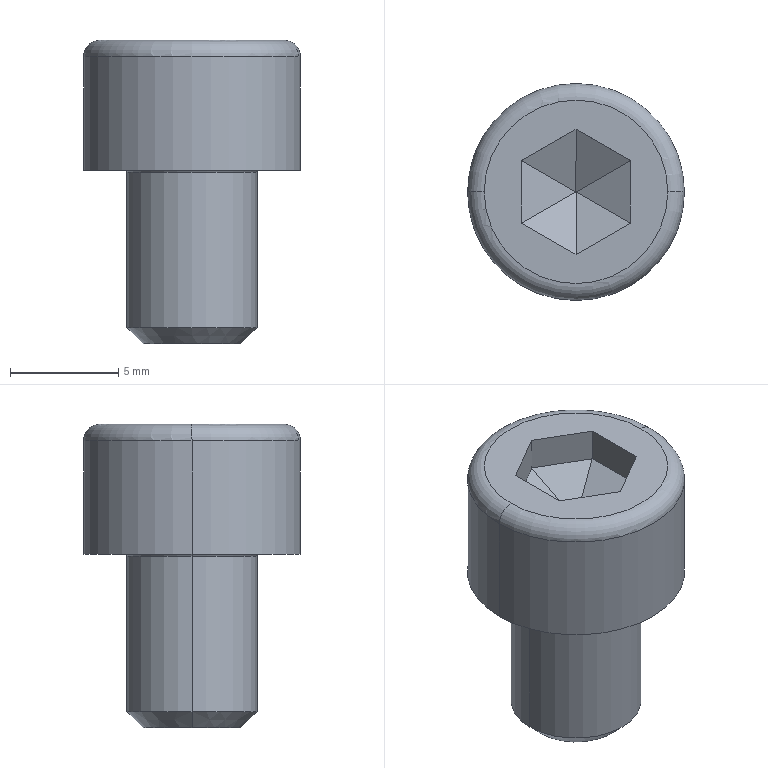Part | SolidWorks | features Chamfer 2, Fillet 2, ICE 2, Extrusion 1, RefAxis 1 | 1 solid | 26 faces | box 10 x 10 x 14 mm | volume 644.591 mm3 | plane 16 | torus 4 | cylinder 4 | cone 2 | commonest cylinder face diameters 6 x2 10 x2
STEP:
#1=CARTESIAN_POINT('',(-3.1,0.,0.));
#2=VERTEX_POINT('',#1);
#3=CARTESIAN_POINT('',(3.1,0.,0.));
#4=VERTEX_POINT('',#3);
#5=CARTESIAN_POINT('',(0.,0.,0.));
#6=DIRECTION('',(0.,0.,1.));
#7=DIRECTION('',(1.,0.,0.));
#8=AXIS2_PLACEMENT_3D('',#5,#6,#7);
#9=CIRCLE('',#8,3.1);
#10=EDGE_CURVE('',#2,#4,#9,.T.);
#11=ORIENTED_EDGE('',*,*,#10,.F.);
#12=CARTESIAN_POINT('',(-3.,0.,-0.1));
#13=VERTEX_POINT('',#12);
#14=CARTESIAN_POINT('',(-3.1,0.,-0.1));
#15=DIRECTION('',(0.,1.,0.));
#16=DIRECTION('',(-1.,0.,0.));
#17=AXIS2_PLACEMENT_3D('',#14,#15,#16);
#18=CIRCLE('',#17,0.1);
#19=EDGE_CURVE('',#2,#13,#18,.T.);
#20=ORIENTED_EDGE('',*,*,#19,.T.);
#21=CARTESIAN_POINT('',(3.,0.,-0.1));
#22=VERTEX_POINT('',#21);
#23=CARTESIAN_POINT('',(0.,0.,-0.1));
#24=DIRECTION('',(0.,0.,-1.));
#25=DIRECTION('',(1.,0.,0.));
#26=AXIS2_PLACEMENT_3D('',#23,#24,#25);
#27=CIRCLE('',#26,3.);
#28=EDGE_CURVE('',#22,#13,#27,.T.);
#29=ORIENTED_EDGE('',*,*,#28,.F.);
#30=CARTESIAN_POINT('',(3.1,0.,-0.1));
#31=DIRECTION('',(0.,-1.,0.));
#32=DIRECTION('',(0.,0.,-1.));
#33=AXIS2_PLACEMENT_3D('',#30,#31,#32);
#34=CIRCLE('',#33,0.1);
#35=EDGE_CURVE('',#4,#22,#34,.T.);
#36=ORIENTED_EDGE('',*,*,#35,.F.);
#37=EDGE_LOOP('',(#11,#20,#29,#36));
#38=FACE_OUTER_BOUND('',#37,.T.);
#39=CARTESIAN_POINT('',(0.,0.,-0.1));
#40=DIRECTION('',(0.,0.,1.));
#41=DIRECTION('',(1.,0.,0.));
#42=AXIS2_PLACEMENT_3D('',#39,#40,#41);
#43=TOROIDAL_SURFACE('',#42,3.1,0.1);
#44=ADVANCED_FACE('',(#38),#43,.F.);
#45=CARTESIAN_POINT('',(-5.,0.,5.231));
#46=VERTEX_POINT('',#45);
#47=CARTESIAN_POINT('',(5.,0.,5.231));
#48=VERTEX_POINT('',#47);
#49=CARTESIAN_POINT('',(0.,0.,5.231));
#50=DIRECTION('',(0.,0.,-1.));
#51=DIRECTION('',(1.,0.,0.));
#52=AXIS2_PLACEMENT_3D('',#49,#50,#51);
#53=CIRCLE('',#52,5.);
#54=EDGE_CURVE('',#46,#48,#53,.T.);
#55=ORIENTED_EDGE('',*,*,#54,.F.);
#56=CARTESIAN_POINT('',(-4.231,0.,6.));
#57=VERTEX_POINT('',#56);
#58=CARTESIAN_POINT('',(-4.231,0.,5.231));
#59=DIRECTION('',(0.,1.,0.));
#60=DIRECTION('',(-1.,0.,0.));
#61=AXIS2_PLACEMENT_3D('',#58,#59,#60);
#62=CIRCLE('',#61,0.7692);
#63=EDGE_CURVE('',#46,#57,#62,.T.);
#64=ORIENTED_EDGE('',*,*,#63,.T.);
#65=CARTESIAN_POINT('',(4.231,0.,6.));
#66=VERTEX_POINT('',#65);
#67=CARTESIAN_POINT('',(0.,0.,6.));
#68=DIRECTION('',(0.,0.,1.));
#69=DIRECTION('',(1.,0.,0.));
#70=AXIS2_PLACEMENT_3D('',#67,#68,#69);
#71=CIRCLE('',#70,4.231);
#72=EDGE_CURVE('',#66,#57,#71,.T.);
#73=ORIENTED_EDGE('',*,*,#72,.F.);
#74=CARTESIAN_POINT('',(4.231,0.,5.231));
#75=DIRECTION('',(0.,-1.,0.));
#76=DIRECTION('',(0.,0.,-1.));
#77=AXIS2_PLACEMENT_3D('',#74,#75,#76);
#78=CIRCLE('',#77,0.7692);
#79=EDGE_CURVE('',#48,#66,#78,.T.);
#80=ORIENTED_EDGE('',*,*,#79,.F.);
#81=EDGE_LOOP('',(#55,#64,#73,#80));
#82=FACE_OUTER_BOUND('',#81,.T.);
#83=CARTESIAN_POINT('',(0.,0.,5.231));
#84=DIRECTION('',(0.,0.,1.));
#85=DIRECTION('',(1.,0.,0.));
#86=AXIS2_PLACEMENT_3D('',#83,#84,#85);
#87=TOROIDAL_SURFACE('',#86,4.231,0.7692);
#88=ADVANCED_FACE('',(#82),#87,.T.);
#89=CARTESIAN_POINT('',(-2.25,0.,-8.));
#90=VERTEX_POINT('',#89);
#91=CARTESIAN_POINT('',(2.25,0.,-8.));
#92=VERTEX_POINT('',#91);
#93=CARTESIAN_POINT('',(0.,0.,-8.));
#94=DIRECTION('',(0.,0.,-1.));
#95=DIRECTION('',(-1.,0.,0.));
#96=AXIS2_PLACEMENT_3D('',#93,#94,#95);
#97=CIRCLE('',#96,2.25);
#98=EDGE_CURVE('',#90,#92,#97,.T.);
#99=ORIENTED_EDGE('',*,*,#98,.F.);
#100=CARTESIAN_POINT('',(-3.,0.,-7.25));
#101=VERTEX_POINT('',#100);
#102=CARTESIAN_POINT('',(-2.25,0.,-8.));
#103=DIRECTION('',(-0.7071,0.,0.7071));
#104=VECTOR('',#103,1000.);
#105=LINE('',#102,#104);
#106=EDGE_CURVE('',#90,#101,#105,.T.);
#107=ORIENTED_EDGE('',*,*,#106,.T.);
#108=CARTESIAN_POINT('',(3.,0.,-7.25));
#109=VERTEX_POINT('',#108);
#110=CARTESIAN_POINT('',(0.,0.,-7.25));
#111=DIRECTION('',(0.,0.,1.));
#112=DIRECTION('',(-1.,0.,0.));
#113=AXIS2_PLACEMENT_3D('',#110,#111,#112);
#114=CIRCLE('',#113,3.);
#115=EDGE_CURVE('',#109,#101,#114,.T.);
#116=ORIENTED_EDGE('',*,*,#115,.F.);
#117=CARTESIAN_POINT('',(2.25,0.,-8.));
#118=DIRECTION('',(0.7071,0.,0.7071));
#119=VECTOR('',#118,1000.);
#120=LINE('',#117,#119);
#121=EDGE_CURVE('',#92,#109,#120,.T.);
#122=ORIENTED_EDGE('',*,*,#121,.F.);
#123=EDGE_LOOP('',(#99,#107,#116,#122));
#124=FACE_OUTER_BOUND('',#123,.T.);
#125=CARTESIAN_POINT('',(0.,0.,-8.));
#126=DIRECTION('',(0.,0.,1.));
#127=DIRECTION('',(1.,0.,0.));
#128=AXIS2_PLACEMENT_3D('',#125,#126,#127);
#129=CONICAL_SURFACE('',#128,2.25,0.7854);
#130=ADVANCED_FACE('',(#124),#129,.T.);
#131=ORIENTED_EDGE('',*,*,#115,.T.);
#132=CARTESIAN_POINT('',(-3.,0.,-8.));
#133=DIRECTION('',(0.,0.,1.));
#134=VECTOR('',#133,1000.);
#135=LINE('',#132,#134);
#136=EDGE_CURVE('',#101,#13,#135,.T.);
#137=ORIENTED_EDGE('',*,*,#136,.T.);
#138=CARTESIAN_POINT('',(0.,0.,-0.1));
#139=DIRECTION('',(0.,0.,-1.));
#140=DIRECTION('',(1.,0.,0.));
#141=AXIS2_PLACEMENT_3D('',#138,#139,#140);
#142=CIRCLE('',#141,3.);
#143=EDGE_CURVE('',#13,#22,#142,.T.);
#144=ORIENTED_EDGE('',*,*,#143,.T.);
#145=CARTESIAN_POINT('',(3.,0.,-8.));
#146=DIRECTION('',(0.,0.,1.));
#147=VECTOR('',#146,1000.);
#148=LINE('',#145,#147);
#149=EDGE_CURVE('',#109,#22,#148,.T.);
#150=ORIENTED_EDGE('',*,*,#149,.F.);
#151=EDGE_LOOP('',(#131,#137,#144,#150));
#152=FACE_OUTER_BOUND('',#151,.T.);
#153=CARTESIAN_POINT('',(0.,0.,-8.));
#154=DIRECTION('',(0.,0.,1.));
#155=DIRECTION('',(1.,0.,0.));
#156=AXIS2_PLACEMENT_3D('',#153,#154,#155);
#157=CYLINDRICAL_SURFACE('',#156,3.);
#158=ADVANCED_FACE('',(#152),#157,.T.);
#159=ORIENTED_EDGE('',*,*,#54,.T.);
#160=CARTESIAN_POINT('',(5.,0.,0.));
#161=VERTEX_POINT('',#160);
#162=CARTESIAN_POINT('',(5.,0.,6.));
#163=DIRECTION('',(0.,0.,-1.));
#164=VECTOR('',#163,1000.);
#165=LINE('',#162,#164);
#166=EDGE_CURVE('',#48,#161,#165,.T.);
#167=ORIENTED_EDGE('',*,*,#166,.T.);
#168=CARTESIAN_POINT('',(-5.,0.,0.));
#169=VERTEX_POINT('',#168);
#170=CARTESIAN_POINT('',(0.,0.,0.));
#171=DIRECTION('',(0.,0.,1.));
#172=DIRECTION('',(1.,0.,0.));
#173=AXIS2_PLACEMENT_3D('',#170,#171,#172);
#174=CIRCLE('',#173,5.);
#175=EDGE_CURVE('',#161,#169,#174,.T.);
#176=ORIENTED_EDGE('',*,*,#175,.T.);
#177=CARTESIAN_POINT('',(-5.,0.,6.));
#178=DIRECTION('',(0.,0.,-1.));
#179=VECTOR('',#178,1000.);
#180=LINE('',#177,#179);
#181=EDGE_CURVE('',#46,#169,#180,.T.);
#182=ORIENTED_EDGE('',*,*,#181,.F.);
#183=EDGE_LOOP('',(#159,#167,#176,#182));
#184=FACE_OUTER_BOUND('',#183,.T.);
#185=CARTESIAN_POINT('',(0.,0.,6.));
#186=DIRECTION('',(0.,0.,-1.));
#187=DIRECTION('',(-1.,0.,0.));
#188=AXIS2_PLACEMENT_3D('',#185,#186,#187);
#189=CYLINDRICAL_SURFACE('',#188,5.);
#190=ADVANCED_FACE('',(#184),#189,.T.);
#191=CARTESIAN_POINT('',(0.,0.,0.));
#192=DIRECTION('',(0.,0.,1.));
#193=DIRECTION('',(1.,0.,0.));
#194=AXIS2_PLACEMENT_3D('',#191,#192,#193);
#195=CIRCLE('',#194,3.1);
#196=EDGE_CURVE('',#4,#2,#195,.T.);
#197=ORIENTED_EDGE('',*,*,#196,.T.);
#198=ORIENTED_EDGE('',*,*,#10,.T.);
#199=EDGE_LOOP('',(#197,#198));
#200=FACE_BOUND('',#199,.T.);
#201=CARTESIAN_POINT('',(0.,0.,0.));
#202=DIRECTION('',(0.,0.,1.));
#203=DIRECTION('',(1.,0.,0.));
#204=AXIS2_PLACEMENT_3D('',#201,#202,#203);
#205=CIRCLE('',#204,5.);
#206=EDGE_CURVE('',#169,#161,#205,.T.);
#207=ORIENTED_EDGE('',*,*,#206,.F.);
#208=ORIENTED_EDGE('',*,*,#175,.F.);
#209=EDGE_LOOP('',(#207,#208));
#210=FACE_OUTER_BOUND('',#209,.T.);
#211=CARTESIAN_POINT('',(0.,0.,0.));
#212=DIRECTION('',(0.,0.,1.));
#213=DIRECTION('',(1.,0.,0.));
#214=AXIS2_PLACEMENT_3D('',#211,#212,#213);
#215=PLANE('',#214);
#216=ADVANCED_FACE('',(#200,#210),#215,.F.);
#217=ORIENTED_EDGE('',*,*,#166,.F.);
#218=CARTESIAN_POINT('',(0.,0.,5.231));
#219=DIRECTION('',(0.,0.,-1.));
#220=DIRECTION('',(1.,0.,0.));
#221=AXIS2_PLACEMENT_3D('',#218,#219,#220);
#222=CIRCLE('',#221,5.);
#223=EDGE_CURVE('',#48,#46,#222,.T.);
#224=ORIENTED_EDGE('',*,*,#223,.T.);
#225=ORIENTED_EDGE('',*,*,#181,.T.);
#226=ORIENTED_EDGE('',*,*,#206,.T.);
#227=EDGE_LOOP('',(#217,#224,#225,#226));
#228=FACE_OUTER_BOUND('',#227,.T.);
#229=CARTESIAN_POINT('',(0.,0.,6.));
#230=DIRECTION('',(0.,0.,-1.));
#231=DIRECTION('',(-1.,0.,0.));
#232=AXIS2_PLACEMENT_3D('',#229,#230,#231);
#233=CYLINDRICAL_SURFACE('',#232,5.);
#234=ADVANCED_FACE('',(#228),#233,.T.);
#235=ORIENTED_EDGE('',*,*,#72,.T.);
#236=CARTESIAN_POINT('',(0.,0.,6.));
#237=DIRECTION('',(0.,0.,1.));
#238=DIRECTION('',(1.,0.,0.));
#239=AXIS2_PLACEMENT_3D('',#236,#237,#238);
#240=CIRCLE('',#239,4.231);
#241=EDGE_CURVE('',#57,#66,#240,.T.);
#242=ORIENTED_EDGE('',*,*,#241,.T.);
#243=EDGE_LOOP('',(#235,#242));
#244=FACE_OUTER_BOUND('',#243,.T.);
#245=CARTESIAN_POINT('',(2.5,-1.443,6.));
#246=VERTEX_POINT('',#245);
#247=CARTESIAN_POINT('',(2.5,1.443,6.));
#248=VERTEX_POINT('',#247);
#249=CARTESIAN_POINT('',(2.5,-1.443,6.));
#250=DIRECTION('',(0.,1.,0.));
#251=VECTOR('',#250,1000.);
#252=LINE('',#249,#251);
#253=EDGE_CURVE('',#246,#248,#252,.T.);
#254=ORIENTED_EDGE('',*,*,#253,.F.);
#255=CARTESIAN_POINT('',(0.,-2.887,6.));
#256=VERTEX_POINT('',#255);
#257=CARTESIAN_POINT('',(0.,-2.887,6.));
#258=DIRECTION('',(0.866,0.5,0.));
#259=VECTOR('',#258,1000.);
#260=LINE('',#257,#259);
#261=EDGE_CURVE('',#256,#246,#260,.T.);
#262=ORIENTED_EDGE('',*,*,#261,.F.);
#263=CARTESIAN_POINT('',(-2.5,-1.443,6.));
#264=VERTEX_POINT('',#263);
#265=CARTESIAN_POINT('',(-2.5,-1.443,6.));
#266=DIRECTION('',(0.866,-0.5,0.));
#267=VECTOR('',#266,1000.);
#268=LINE('',#265,#267);
#269=EDGE_CURVE('',#264,#256,#268,.T.);
#270=ORIENTED_EDGE('',*,*,#269,.F.);
#271=CARTESIAN_POINT('',(-2.5,1.443,6.));
#272=VERTEX_POINT('',#271);
#273=CARTESIAN_POINT('',(-2.5,1.443,6.));
#274=DIRECTION('',(0.,-1.,0.));
#275=VECTOR('',#274,1000.);
#276=LINE('',#273,#275);
#277=EDGE_CURVE('',#272,#264,#276,.T.);
#278=ORIENTED_EDGE('',*,*,#277,.F.);
#279=CARTESIAN_POINT('',(0.,2.887,6.));
#280=VERTEX_POINT('',#279);
#281=CARTESIAN_POINT('',(0.,2.887,6.));
#282=DIRECTION('',(-0.866,-0.5,0.));
#283=VECTOR('',#282,1000.);
#284=LINE('',#281,#283);
#285=EDGE_CURVE('',#280,#272,#284,.T.);
#286=ORIENTED_EDGE('',*,*,#285,.F.);
#287=CARTESIAN_POINT('',(2.5,1.443,6.));
#288=DIRECTION('',(-0.866,0.5,0.));
#289=VECTOR('',#288,1000.);
#290=LINE('',#287,#289);
#291=EDGE_CURVE('',#248,#280,#290,.T.);
#292=ORIENTED_EDGE('',*,*,#291,.F.);
#293=EDGE_LOOP('',(#254,#262,#270,#278,#286,#292));
#294=FACE_BOUND('',#293,.T.);
#295=CARTESIAN_POINT('',(0.,0.,6.));
#296=DIRECTION('',(0.,0.,1.));
#297=DIRECTION('',(1.,0.,0.));
#298=AXIS2_PLACEMENT_3D('',#295,#296,#297);
#299=PLANE('',#298);
#300=ADVANCED_FACE('',(#244,#294),#299,.T.);
#301=CARTESIAN_POINT('',(2.5,1.443,4.441));
#302=VERTEX_POINT('',#301);
#303=CARTESIAN_POINT('',(2.5,1.443,3.));
#304=DIRECTION('',(0.,0.,1.));
#305=VECTOR('',#304,1000.);
#306=LINE('',#303,#305);
#307=EDGE_CURVE('',#302,#248,#306,.T.);
#308=ORIENTED_EDGE('',*,*,#307,.F.);
#309=CARTESIAN_POINT('',(2.5,-1.443,4.441));
#310=VERTEX_POINT('',#309);
#311=CARTESIAN_POINT('',(2.5,-1.443,4.441));
#312=DIRECTION('',(0.,-1.,0.));
#313=VECTOR('',#312,1000.);
#314=LINE('',#311,#313);
#315=EDGE_CURVE('',#302,#310,#314,.T.);
#316=ORIENTED_EDGE('',*,*,#315,.T.);
#317=CARTESIAN_POINT('',(2.5,-1.443,3.));
#318=DIRECTION('',(0.,0.,1.));
#319=VECTOR('',#318,1000.);
#320=LINE('',#317,#319);
#321=EDGE_CURVE('',#310,#246,#320,.T.);
#322=ORIENTED_EDGE('',*,*,#321,.T.);
#323=ORIENTED_EDGE('',*,*,#253,.T.);
#324=EDGE_LOOP('',(#308,#316,#322,#323));
#325=FACE_OUTER_BOUND('',#324,.T.);
#326=CARTESIAN_POINT('',(2.5,-1.443,3.));
#327=DIRECTION('',(1.,0.,0.));
#328=DIRECTION('',(0.,0.,-1.));
#329=AXIS2_PLACEMENT_3D('',#326,#327,#328);
#330=PLANE('',#329);
#331=ADVANCED_FACE('',(#325),#330,.F.);
#332=ORIENTED_EDGE('',*,*,#321,.F.);
#333=CARTESIAN_POINT('',(0.,-2.887,4.441));
#334=VERTEX_POINT('',#333);
#335=CARTESIAN_POINT('',(0.,-2.887,4.441));
#336=DIRECTION('',(-0.866,-0.5,0.));
#337=VECTOR('',#336,1000.);
#338=LINE('',#335,#337);
#339=EDGE_CURVE('',#310,#334,#338,.T.);
#340=ORIENTED_EDGE('',*,*,#339,.T.);
#341=CARTESIAN_POINT('',(0.,-2.887,3.));
#342=DIRECTION('',(0.,0.,1.));
#343=VECTOR('',#342,1000.);
#344=LINE('',#341,#343);
#345=EDGE_CURVE('',#334,#256,#344,.T.);
#346=ORIENTED_EDGE('',*,*,#345,.T.);
#347=ORIENTED_EDGE('',*,*,#261,.T.);
#348=EDGE_LOOP('',(#332,#340,#346,#347));
#349=FACE_OUTER_BOUND('',#348,.T.);
#350=CARTESIAN_POINT('',(0.,-2.887,3.));
#351=DIRECTION('',(0.5,-0.866,0.));
#352=DIRECTION('',(0.866,0.5,0.));
#353=AXIS2_PLACEMENT_3D('',#350,#351,#352);
#354=PLANE('',#353);
#355=ADVANCED_FACE('',(#349),#354,.F.);
#356=ORIENTED_EDGE('',*,*,#345,.F.);
#357=CARTESIAN_POINT('',(-2.5,-1.443,4.441));
#358=VERTEX_POINT('',#357);
#359=CARTESIAN_POINT('',(-2.5,-1.443,4.441));
#360=DIRECTION('',(-0.866,0.5,0.));
#361=VECTOR('',#360,1000.);
#362=LINE('',#359,#361);
#363=EDGE_CURVE('',#334,#358,#362,.T.);
#364=ORIENTED_EDGE('',*,*,#363,.T.);
#365=CARTESIAN_POINT('',(-2.5,-1.443,3.));
#366=DIRECTION('',(0.,0.,1.));
#367=VECTOR('',#366,1000.);
#368=LINE('',#365,#367);
#369=EDGE_CURVE('',#358,#264,#368,.T.);
#370=ORIENTED_EDGE('',*,*,#369,.T.);
#371=ORIENTED_EDGE('',*,*,#269,.T.);
#372=EDGE_LOOP('',(#356,#364,#370,#371));
#373=FACE_OUTER_BOUND('',#372,.T.);
#374=CARTESIAN_POINT('',(-2.5,-1.443,3.));
#375=DIRECTION('',(-0.5,-0.866,0.));
#376=DIRECTION('',(0.866,-0.5,0.));
#377=AXIS2_PLACEMENT_3D('',#374,#375,#376);
#378=PLANE('',#377);
#379=ADVANCED_FACE('',(#373),#378,.F.);
#380=ORIENTED_EDGE('',*,*,#369,.F.);
#381=CARTESIAN_POINT('',(-2.5,1.443,4.441));
#382=VERTEX_POINT('',#381);
#383=CARTESIAN_POINT('',(-2.5,1.443,4.441));
#384=DIRECTION('',(0.,1.,0.));
#385=VECTOR('',#384,1000.);
#386=LINE('',#383,#385);
#387=EDGE_CURVE('',#358,#382,#386,.T.);
#388=ORIENTED_EDGE('',*,*,#387,.T.);
#389=CARTESIAN_POINT('',(-2.5,1.443,3.));
#390=DIRECTION('',(0.,0.,1.));
#391=VECTOR('',#390,1000.);
#392=LINE('',#389,#391);
#393=EDGE_CURVE('',#382,#272,#392,.T.);
#394=ORIENTED_EDGE('',*,*,#393,.T.);
#395=ORIENTED_EDGE('',*,*,#277,.T.);
#396=EDGE_LOOP('',(#380,#388,#394,#395));
#397=FACE_OUTER_BOUND('',#396,.T.);
#398=CARTESIAN_POINT('',(-2.5,1.443,3.));
#399=DIRECTION('',(-1.,0.,0.));
#400=DIRECTION('',(0.,0.,1.));
#401=AXIS2_PLACEMENT_3D('',#398,#399,#400);
#402=PLANE('',#401);
#403=ADVANCED_FACE('',(#397),#402,.F.);
#404=ORIENTED_EDGE('',*,*,#393,.F.);
#405=CARTESIAN_POINT('',(0.,2.887,4.441));
#406=VERTEX_POINT('',#405);
#407=CARTESIAN_POINT('',(0.,2.887,4.441));
#408=DIRECTION('',(0.866,0.5,0.));
#409=VECTOR('',#408,1000.);
#410=LINE('',#407,#409);
#411=EDGE_CURVE('',#382,#406,#410,.T.);
#412=ORIENTED_EDGE('',*,*,#411,.T.);
#413=CARTESIAN_POINT('',(0.,2.887,3.));
#414=DIRECTION('',(0.,0.,1.));
#415=VECTOR('',#414,1000.);
#416=LINE('',#413,#415);
#417=EDGE_CURVE('',#406,#280,#416,.T.);
#418=ORIENTED_EDGE('',*,*,#417,.T.);
#419=ORIENTED_EDGE('',*,*,#285,.T.);
#420=EDGE_LOOP('',(#404,#412,#418,#419));
#421=FACE_OUTER_BOUND('',#420,.T.);
#422=CARTESIAN_POINT('',(0.,2.887,3.));
#423=DIRECTION('',(-0.5,0.866,0.));
#424=DIRECTION('',(-0.866,-0.5,0.));
#425=AXIS2_PLACEMENT_3D('',#422,#423,#424);
#426=PLANE('',#425);
#427=ADVANCED_FACE('',(#421),#426,.F.);
#428=ORIENTED_EDGE('',*,*,#417,.F.);
#429=CARTESIAN_POINT('',(2.5,1.443,4.441));
#430=DIRECTION('',(0.866,-0.5,0.));
#431=VECTOR('',#430,1000.);
#432=LINE('',#429,#431);
#433=EDGE_CURVE('',#406,#302,#432,.T.);
#434=ORIENTED_EDGE('',*,*,#433,.T.);
#435=ORIENTED_EDGE('',*,*,#307,.T.);
#436=ORIENTED_EDGE('',*,*,#291,.T.);
#437=EDGE_LOOP('',(#428,#434,#435,#436));
#438=FACE_OUTER_BOUND('',#437,.T.);
#439=CARTESIAN_POINT('',(2.5,1.443,3.));
#440=DIRECTION('',(0.5,0.866,0.));
#441=DIRECTION('',(-0.866,0.5,0.));
#442=AXIS2_PLACEMENT_3D('',#439,#440,#441);
#443=PLANE('',#442);
#444=ADVANCED_FACE('',(#438),#443,.F.);
#445=CARTESIAN_POINT('',(0.,0.004907,3.));
#446=VERTEX_POINT('',#445);
#447=CARTESIAN_POINT('',(-0.00425,0.002453,3.));
#448=VERTEX_POINT('',#447);
#449=CARTESIAN_POINT('',(-0.002125,0.00368,3.));
#450=DIRECTION('',(-0.866,-0.5,0.));
#451=VECTOR('',#450,1000.);
#452=LINE('',#449,#451);
#453=EDGE_CURVE('',#446,#448,#452,.T.);
#454=ORIENTED_EDGE('',*,*,#453,.T.);
#455=CARTESIAN_POINT('',(-0.00425,-0.002453,3.));
#456=VERTEX_POINT('',#455);
#457=CARTESIAN_POINT('',(-0.00425,0.,3.));
#458=DIRECTION('',(0.,-1.,0.));
#459=VECTOR('',#458,1000.);
#460=LINE('',#457,#459);
#461=EDGE_CURVE('',#448,#456,#460,.T.);
#462=ORIENTED_EDGE('',*,*,#461,.T.);
#463=CARTESIAN_POINT('',(0.,-0.004907,3.));
#464=VERTEX_POINT('',#463);
#465=CARTESIAN_POINT('',(-0.002125,-0.00368,3.));
#466=DIRECTION('',(0.866,-0.5,0.));
#467=VECTOR('',#466,1000.);
#468=LINE('',#465,#467);
#469=EDGE_CURVE('',#456,#464,#468,.T.);
#470=ORIENTED_EDGE('',*,*,#469,.T.);
#471=CARTESIAN_POINT('',(0.00425,-0.002453,3.));
#472=VERTEX_POINT('',#471);
#473=CARTESIAN_POINT('',(0.002125,-0.00368,3.));
#474=DIRECTION('',(0.866,0.5,0.));
#475=VECTOR('',#474,1000.);
#476=LINE('',#473,#475);
#477=EDGE_CURVE('',#464,#472,#476,.T.);
#478=ORIENTED_EDGE('',*,*,#477,.T.);
#479=CARTESIAN_POINT('',(0.00425,0.002453,3.));
#480=VERTEX_POINT('',#479);
#481=CARTESIAN_POINT('',(0.00425,0.,3.));
#482=DIRECTION('',(0.,1.,0.));
#483=VECTOR('',#482,1000.);
#484=LINE('',#481,#483);
#485=EDGE_CURVE('',#472,#480,#484,.T.);
#486=ORIENTED_EDGE('',*,*,#485,.T.);
#487=CARTESIAN_POINT('',(0.002125,0.00368,3.));
#488=DIRECTION('',(-0.866,0.5,0.));
#489=VECTOR('',#488,1000.);
#490=LINE('',#487,#489);
#491=EDGE_CURVE('',#480,#446,#490,.T.);
#492=ORIENTED_EDGE('',*,*,#491,.T.);
#493=EDGE_LOOP('',(#454,#462,#470,#478,#486,#492));
#494=FACE_OUTER_BOUND('',#493,.T.);
#495=CARTESIAN_POINT('',(0.,0.,3.));
#496=DIRECTION('',(0.,0.,1.));
#497=DIRECTION('',(1.,0.,0.));
#498=AXIS2_PLACEMENT_3D('',#495,#496,#497);
#499=PLANE('',#498);
#500=ADVANCED_FACE('',(#494),#499,.T.);
#501=ORIENTED_EDGE('',*,*,#136,.F.);
#502=CARTESIAN_POINT('',(0.,0.,-7.25));
#503=DIRECTION('',(0.,0.,1.));
#504=DIRECTION('',(-1.,0.,0.));
#505=AXIS2_PLACEMENT_3D('',#502,#503,#504);
#506=CIRCLE('',#505,3.);
#507=EDGE_CURVE('',#101,#109,#506,.T.);
#508=ORIENTED_EDGE('',*,*,#507,.T.);
#509=ORIENTED_EDGE('',*,*,#149,.T.);
#510=ORIENTED_EDGE('',*,*,#28,.T.);
#511=EDGE_LOOP('',(#501,#508,#509,#510));
#512=FACE_OUTER_BOUND('',#511,.T.);
#513=CARTESIAN_POINT('',(0.,0.,-8.));
#514=DIRECTION('',(0.,0.,1.));
#515=DIRECTION('',(1.,0.,0.));
#516=AXIS2_PLACEMENT_3D('',#513,#514,#515);
#517=CYLINDRICAL_SURFACE('',#516,3.);
#518=ADVANCED_FACE('',(#512),#517,.T.);
#519=CARTESIAN_POINT('',(0.,0.,-8.));
#520=DIRECTION('',(0.,0.,-1.));
#521=DIRECTION('',(-1.,0.,0.));
#522=AXIS2_PLACEMENT_3D('',#519,#520,#521);
#523=CIRCLE('',#522,2.25);
#524=EDGE_CURVE('',#92,#90,#523,.T.);
#525=ORIENTED_EDGE('',*,*,#524,.T.);
#526=ORIENTED_EDGE('',*,*,#98,.T.);
#527=EDGE_LOOP('',(#525,#526));
#528=FACE_OUTER_BOUND('',#527,.T.);
#529=CARTESIAN_POINT('',(0.,0.,-8.));
#530=DIRECTION('',(0.,0.,-1.));
#531=DIRECTION('',(-1.,0.,0.));
#532=AXIS2_PLACEMENT_3D('',#529,#530,#531);
#533=PLANE('',#532);
#534=ADVANCED_FACE('',(#528),#533,.T.);
#535=ORIENTED_EDGE('',*,*,#106,.F.);
#536=ORIENTED_EDGE('',*,*,#524,.F.);
#537=ORIENTED_EDGE('',*,*,#121,.T.);
#538=ORIENTED_EDGE('',*,*,#507,.F.);
#539=EDGE_LOOP('',(#535,#536,#537,#538));
#540=FACE_OUTER_BOUND('',#539,.T.);
#541=CARTESIAN_POINT('',(0.,0.,-8.));
#542=DIRECTION('',(0.,0.,1.));
#543=DIRECTION('',(1.,0.,0.));
#544=AXIS2_PLACEMENT_3D('',#541,#542,#543);
#545=CONICAL_SURFACE('',#544,2.25,0.7854);
#546=ADVANCED_FACE('',(#540),#545,.T.);
#547=ORIENTED_EDGE('',*,*,#63,.F.);
#548=ORIENTED_EDGE('',*,*,#223,.F.);
#549=ORIENTED_EDGE('',*,*,#79,.T.);
#550=ORIENTED_EDGE('',*,*,#241,.F.);
#551=EDGE_LOOP('',(#547,#548,#549,#550));
#552=FACE_OUTER_BOUND('',#551,.T.);
#553=CARTESIAN_POINT('',(0.,0.,5.231));
#554=DIRECTION('',(0.,0.,1.));
#555=DIRECTION('',(1.,0.,0.));
#556=AXIS2_PLACEMENT_3D('',#553,#554,#555);
#557=TOROIDAL_SURFACE('',#556,4.231,0.7692);
#558=ADVANCED_FACE('',(#552),#557,.T.);
#559=CARTESIAN_POINT('',(0.0034,-0.001963,3.));
#560=DIRECTION('',(-0.7746,0.4472,-0.4472));
#561=VECTOR('',#560,1000.);
#562=LINE('',#559,#561);
#563=EDGE_CURVE('',#310,#472,#562,.T.);
#564=ORIENTED_EDGE('',*,*,#563,.F.);
#565=ORIENTED_EDGE('',*,*,#315,.F.);
#566=CARTESIAN_POINT('',(0.0034,0.001963,3.));
#567=DIRECTION('',(0.7746,0.4472,0.4472));
#568=VECTOR('',#567,1000.);
#569=LINE('',#566,#568);
#570=EDGE_CURVE('',#480,#302,#569,.T.);
#571=ORIENTED_EDGE('',*,*,#570,.F.);
#572=ORIENTED_EDGE('',*,*,#485,.F.);
#573=EDGE_LOOP('',(#564,#565,#571,#572));
#574=FACE_OUTER_BOUND('',#573,.T.);
#575=CARTESIAN_POINT('',(0.00425,0.,3.));
#576=DIRECTION('',(0.5,0.,-0.866));
#577=DIRECTION('',(0.,1.,0.));
#578=AXIS2_PLACEMENT_3D('',#575,#576,#577);
#579=PLANE('',#578);
#580=ADVANCED_FACE('',(#574),#579,.F.);
#581=ORIENTED_EDGE('',*,*,#570,.T.);
#582=ORIENTED_EDGE('',*,*,#433,.F.);
#583=CARTESIAN_POINT('',(0.,0.003926,3.));
#584=DIRECTION('',(0.,0.8944,0.4472));
#585=VECTOR('',#584,1000.);
#586=LINE('',#583,#585);
#587=EDGE_CURVE('',#446,#406,#586,.T.);
#588=ORIENTED_EDGE('',*,*,#587,.F.);
#589=ORIENTED_EDGE('',*,*,#491,.F.);
#590=EDGE_LOOP('',(#581,#582,#588,#589));
#591=FACE_OUTER_BOUND('',#590,.T.);
#592=CARTESIAN_POINT('',(0.002125,0.00368,3.));
#593=DIRECTION('',(0.25,0.433,-0.866));
#594=DIRECTION('',(-0.866,0.5,0.));
#595=AXIS2_PLACEMENT_3D('',#592,#593,#594);
#596=PLANE('',#595);
#597=ADVANCED_FACE('',(#591),#596,.F.);
#598=ORIENTED_EDGE('',*,*,#563,.T.);
#599=ORIENTED_EDGE('',*,*,#477,.F.);
#600=CARTESIAN_POINT('',(0.,-0.003926,3.));
#601=DIRECTION('',(0.,0.8944,-0.4472));
#602=VECTOR('',#601,1000.);
#603=LINE('',#600,#602);
#604=EDGE_CURVE('',#334,#464,#603,.T.);
#605=ORIENTED_EDGE('',*,*,#604,.F.);
#606=ORIENTED_EDGE('',*,*,#339,.F.);
#607=EDGE_LOOP('',(#598,#599,#605,#606));
#608=FACE_OUTER_BOUND('',#607,.T.);
#609=CARTESIAN_POINT('',(0.002125,-0.00368,3.));
#610=DIRECTION('',(0.25,-0.433,-0.866));
#611=DIRECTION('',(0.866,0.5,0.));
#612=AXIS2_PLACEMENT_3D('',#609,#610,#611);
#613=PLANE('',#612);
#614=ADVANCED_FACE('',(#608),#613,.F.);
#615=ORIENTED_EDGE('',*,*,#587,.T.);
#616=ORIENTED_EDGE('',*,*,#411,.F.);
#617=CARTESIAN_POINT('',(-0.0034,0.001963,3.));
#618=DIRECTION('',(-0.7746,0.4472,0.4472));
#619=VECTOR('',#618,1000.);
#620=LINE('',#617,#619);
#621=EDGE_CURVE('',#448,#382,#620,.T.);
#622=ORIENTED_EDGE('',*,*,#621,.F.);
#623=ORIENTED_EDGE('',*,*,#453,.F.);
#624=EDGE_LOOP('',(#615,#616,#622,#623));
#625=FACE_OUTER_BOUND('',#624,.T.);
#626=CARTESIAN_POINT('',(-0.002125,0.00368,3.));
#627=DIRECTION('',(-0.25,0.433,-0.866));
#628=DIRECTION('',(-0.866,-0.5,0.));
#629=AXIS2_PLACEMENT_3D('',#626,#627,#628);
#630=PLANE('',#629);
#631=ADVANCED_FACE('',(#625),#630,.F.);
#632=ORIENTED_EDGE('',*,*,#604,.T.);
#633=ORIENTED_EDGE('',*,*,#469,.F.);
#634=CARTESIAN_POINT('',(-0.0034,-0.001963,3.));
#635=DIRECTION('',(0.7746,0.4472,-0.4472));
#636=VECTOR('',#635,1000.);
#637=LINE('',#634,#636);
#638=EDGE_CURVE('',#358,#456,#637,.T.);
#639=ORIENTED_EDGE('',*,*,#638,.F.);
#640=ORIENTED_EDGE('',*,*,#363,.F.);
#641=EDGE_LOOP('',(#632,#633,#639,#640));
#642=FACE_OUTER_BOUND('',#641,.T.);
#643=CARTESIAN_POINT('',(-0.002125,-0.00368,3.));
#644=DIRECTION('',(-0.25,-0.433,-0.866));
#645=DIRECTION('',(0.866,-0.5,0.));
#646=AXIS2_PLACEMENT_3D('',#643,#644,#645);
#647=PLANE('',#646);
#648=ADVANCED_FACE('',(#642),#647,.F.);
#649=ORIENTED_EDGE('',*,*,#621,.T.);
#650=ORIENTED_EDGE('',*,*,#387,.F.);
#651=ORIENTED_EDGE('',*,*,#638,.T.);
#652=ORIENTED_EDGE('',*,*,#461,.F.);
#653=EDGE_LOOP('',(#649,#650,#651,#652));
#654=FACE_OUTER_BOUND('',#653,.T.);
#655=CARTESIAN_POINT('',(-0.00425,0.,3.));
#656=DIRECTION('',(-0.5,0.,-0.866));
#657=DIRECTION('',(0.,-1.,0.));
#658=AXIS2_PLACEMENT_3D('',#655,#656,#657);
#659=PLANE('',#658);
#660=ADVANCED_FACE('',(#654),#659,.F.);
#661=ORIENTED_EDGE('',*,*,#19,.F.);
#662=ORIENTED_EDGE('',*,*,#196,.F.);
#663=ORIENTED_EDGE('',*,*,#35,.T.);
#664=ORIENTED_EDGE('',*,*,#143,.F.);
#665=EDGE_LOOP('',(#661,#662,#663,#664));
#666=FACE_OUTER_BOUND('',#665,.T.);
#667=CARTESIAN_POINT('',(0.,0.,-0.1));
#668=DIRECTION('',(0.,0.,1.));
#669=DIRECTION('',(1.,0.,0.));
#670=AXIS2_PLACEMENT_3D('',#667,#668,#669);
#671=TOROIDAL_SURFACE('',#670,3.1,0.1);
#672=ADVANCED_FACE('',(#666),#671,.F.);
#673=CLOSED_SHELL('',(#44,#88,#130,#158,#190,#216,#234,#300,#331,#355,#379,#403,#427,#444,#500,#518,#534,#546,#558,#580,#597,#614,#631,#648,#660,#672));
#674=MANIFOLD_SOLID_BREP('',#673);
#675=CARTESIAN_POINT('',(0.,0.,0.));
#676=DIRECTION('',(0.,0.,1.));
#677=DIRECTION('',(1.,0.,0.));
#678=AXIS2_PLACEMENT_3D('',#675,#676,#677);
#679=(LENGTH_UNIT()NAMED_UNIT(*)SI_UNIT(.MILLI.,.METRE.));
#680=UNCERTAINTY_MEASURE_WITH_UNIT(LENGTH_MEASURE(0.00001),#679,'','');
#681=(NAMED_UNIT(*)PLANE_ANGLE_UNIT()SI_UNIT($,.RADIAN.));
#682=(NAMED_UNIT(*)SI_UNIT($,.STERADIAN.)SOLID_ANGLE_UNIT());
#683=(GEOMETRIC_REPRESENTATION_CONTEXT(3)GLOBAL_UNCERTAINTY_ASSIGNED_CONTEXT((#680))GLOBAL_UNIT_ASSIGNED_CONTEXT((#679,#681,#682))REPRESENTATION_CONTEXT('',''));
#684=ADVANCED_BREP_SHAPE_REPRESENTATION('',(#674,#678),#683);